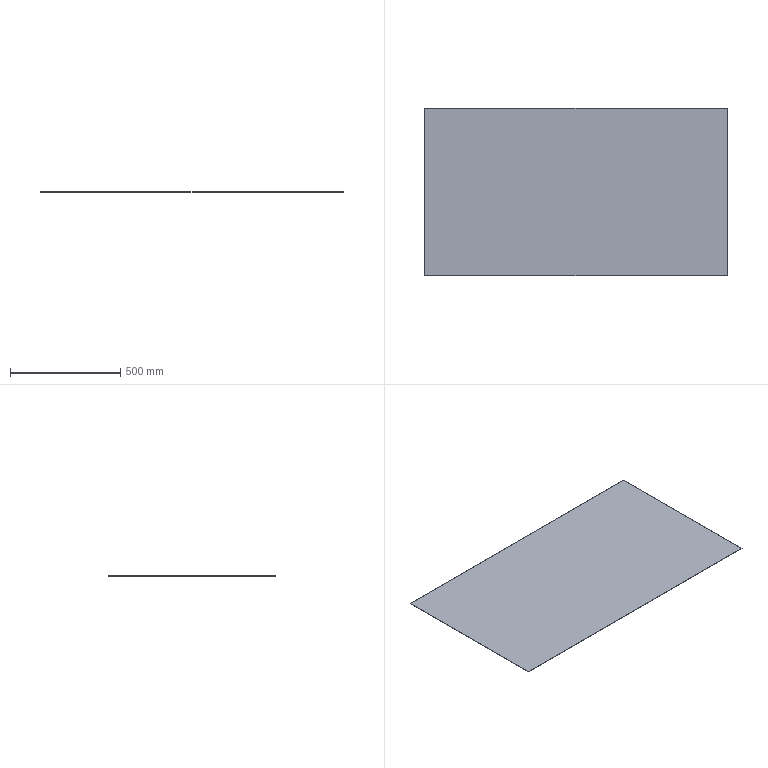Part | SolidWorks | 1 solid | 6 faces | box 1374 x 760 x 1.5 mm | volume 1566360 mm3 | plane 6
STEP:
#1=CARTESIAN_POINT('',(5.,-365.,0.));
#2=VERTEX_POINT('',#1);
#3=CARTESIAN_POINT('',(5.,395.,0.));
#4=VERTEX_POINT('',#3);
#5=CARTESIAN_POINT('',(5.,-365.,0.));
#6=DIRECTION('',(0.,1.,0.));
#7=VECTOR('',#6,1000.);
#8=LINE('',#5,#7);
#9=EDGE_CURVE('',#2,#4,#8,.T.);
#10=ORIENTED_EDGE('',*,*,#9,.T.);
#11=CARTESIAN_POINT('',(5.,395.,1.5));
#12=VERTEX_POINT('',#11);
#13=CARTESIAN_POINT('',(5.,395.,1.5));
#14=DIRECTION('',(0.,0.,-1.));
#15=VECTOR('',#14,1000.);
#16=LINE('',#13,#15);
#17=EDGE_CURVE('',#12,#4,#16,.T.);
#18=ORIENTED_EDGE('',*,*,#17,.F.);
#19=CARTESIAN_POINT('',(5.,-365.,1.5));
#20=VERTEX_POINT('',#19);
#21=CARTESIAN_POINT('',(5.,-365.,1.5));
#22=DIRECTION('',(0.,1.,0.));
#23=VECTOR('',#22,1000.);
#24=LINE('',#21,#23);
#25=EDGE_CURVE('',#20,#12,#24,.T.);
#26=ORIENTED_EDGE('',*,*,#25,.F.);
#27=CARTESIAN_POINT('',(5.,-365.,1.5));
#28=DIRECTION('',(0.,0.,-1.));
#29=VECTOR('',#28,1000.);
#30=LINE('',#27,#29);
#31=EDGE_CURVE('',#20,#2,#30,.T.);
#32=ORIENTED_EDGE('',*,*,#31,.T.);
#33=EDGE_LOOP('',(#10,#18,#26,#32));
#34=FACE_OUTER_BOUND('',#33,.T.);
#35=CARTESIAN_POINT('',(5.,-365.,1.5));
#36=DIRECTION('',(-1.,0.,0.));
#37=DIRECTION('',(0.,0.,1.));
#38=AXIS2_PLACEMENT_3D('',#35,#36,#37);
#39=PLANE('',#38);
#40=ADVANCED_FACE('',(#34),#39,.F.);
#41=CARTESIAN_POINT('',(-1369.,395.,0.));
#42=VERTEX_POINT('',#41);
#43=CARTESIAN_POINT('',(5.,395.,0.));
#44=DIRECTION('',(-1.,0.,0.));
#45=VECTOR('',#44,1000.);
#46=LINE('',#43,#45);
#47=EDGE_CURVE('',#4,#42,#46,.T.);
#48=ORIENTED_EDGE('',*,*,#47,.T.);
#49=CARTESIAN_POINT('',(-1369.,395.,1.5));
#50=VERTEX_POINT('',#49);
#51=CARTESIAN_POINT('',(-1369.,395.,1.5));
#52=DIRECTION('',(0.,0.,-1.));
#53=VECTOR('',#52,1000.);
#54=LINE('',#51,#53);
#55=EDGE_CURVE('',#50,#42,#54,.T.);
#56=ORIENTED_EDGE('',*,*,#55,.F.);
#57=CARTESIAN_POINT('',(5.,395.,1.5));
#58=DIRECTION('',(-1.,0.,0.));
#59=VECTOR('',#58,1000.);
#60=LINE('',#57,#59);
#61=EDGE_CURVE('',#12,#50,#60,.T.);
#62=ORIENTED_EDGE('',*,*,#61,.F.);
#63=ORIENTED_EDGE('',*,*,#17,.T.);
#64=EDGE_LOOP('',(#48,#56,#62,#63));
#65=FACE_OUTER_BOUND('',#64,.T.);
#66=CARTESIAN_POINT('',(5.,395.,1.5));
#67=DIRECTION('',(0.,-1.,0.));
#68=DIRECTION('',(1.,0.,0.));
#69=AXIS2_PLACEMENT_3D('',#66,#67,#68);
#70=PLANE('',#69);
#71=ADVANCED_FACE('',(#65),#70,.F.);
#72=CARTESIAN_POINT('',(-1369.,-365.,0.));
#73=VERTEX_POINT('',#72);
#74=CARTESIAN_POINT('',(-1369.,-365.,0.));
#75=DIRECTION('',(0.,-1.,0.));
#76=VECTOR('',#75,1000.);
#77=LINE('',#74,#76);
#78=EDGE_CURVE('',#42,#73,#77,.T.);
#79=ORIENTED_EDGE('',*,*,#78,.T.);
#80=CARTESIAN_POINT('',(-1369.,-365.,1.5));
#81=VERTEX_POINT('',#80);
#82=CARTESIAN_POINT('',(-1369.,-365.,1.5));
#83=DIRECTION('',(0.,0.,-1.));
#84=VECTOR('',#83,1000.);
#85=LINE('',#82,#84);
#86=EDGE_CURVE('',#81,#73,#85,.T.);
#87=ORIENTED_EDGE('',*,*,#86,.F.);
#88=CARTESIAN_POINT('',(-1369.,-365.,1.5));
#89=DIRECTION('',(0.,-1.,0.));
#90=VECTOR('',#89,1000.);
#91=LINE('',#88,#90);
#92=EDGE_CURVE('',#50,#81,#91,.T.);
#93=ORIENTED_EDGE('',*,*,#92,.F.);
#94=ORIENTED_EDGE('',*,*,#55,.T.);
#95=EDGE_LOOP('',(#79,#87,#93,#94));
#96=FACE_OUTER_BOUND('',#95,.T.);
#97=CARTESIAN_POINT('',(-1369.,-365.,1.5));
#98=DIRECTION('',(1.,0.,0.));
#99=DIRECTION('',(0.,0.,-1.));
#100=AXIS2_PLACEMENT_3D('',#97,#98,#99);
#101=PLANE('',#100);
#102=ADVANCED_FACE('',(#96),#101,.F.);
#103=CARTESIAN_POINT('',(5.,-365.,0.));
#104=DIRECTION('',(1.,0.,0.));
#105=VECTOR('',#104,1000.);
#106=LINE('',#103,#105);
#107=EDGE_CURVE('',#73,#2,#106,.T.);
#108=ORIENTED_EDGE('',*,*,#107,.T.);
#109=ORIENTED_EDGE('',*,*,#31,.F.);
#110=CARTESIAN_POINT('',(5.,-365.,1.5));
#111=DIRECTION('',(1.,0.,0.));
#112=VECTOR('',#111,1000.);
#113=LINE('',#110,#112);
#114=EDGE_CURVE('',#81,#20,#113,.T.);
#115=ORIENTED_EDGE('',*,*,#114,.F.);
#116=ORIENTED_EDGE('',*,*,#86,.T.);
#117=EDGE_LOOP('',(#108,#109,#115,#116));
#118=FACE_OUTER_BOUND('',#117,.T.);
#119=CARTESIAN_POINT('',(5.,-365.,1.5));
#120=DIRECTION('',(0.,1.,0.));
#121=DIRECTION('',(-1.,0.,0.));
#122=AXIS2_PLACEMENT_3D('',#119,#120,#121);
#123=PLANE('',#122);
#124=ADVANCED_FACE('',(#118),#123,.F.);
#125=ORIENTED_EDGE('',*,*,#25,.T.);
#126=ORIENTED_EDGE('',*,*,#61,.T.);
#127=ORIENTED_EDGE('',*,*,#92,.T.);
#128=ORIENTED_EDGE('',*,*,#114,.T.);
#129=EDGE_LOOP('',(#125,#126,#127,#128));
#130=FACE_OUTER_BOUND('',#129,.T.);
#131=CARTESIAN_POINT('',(0.,0.,1.5));
#132=DIRECTION('',(0.,0.,1.));
#133=DIRECTION('',(1.,0.,0.));
#134=AXIS2_PLACEMENT_3D('',#131,#132,#133);
#135=PLANE('',#134);
#136=ADVANCED_FACE('',(#130),#135,.T.);
#137=ORIENTED_EDGE('',*,*,#9,.F.);
#138=ORIENTED_EDGE('',*,*,#107,.F.);
#139=ORIENTED_EDGE('',*,*,#78,.F.);
#140=ORIENTED_EDGE('',*,*,#47,.F.);
#141=EDGE_LOOP('',(#137,#138,#139,#140));
#142=FACE_OUTER_BOUND('',#141,.T.);
#143=CARTESIAN_POINT('',(0.,0.,0.));
#144=DIRECTION('',(0.,0.,1.));
#145=DIRECTION('',(1.,0.,0.));
#146=AXIS2_PLACEMENT_3D('',#143,#144,#145);
#147=PLANE('',#146);
#148=ADVANCED_FACE('',(#142),#147,.F.);
#149=CLOSED_SHELL('',(#40,#71,#102,#124,#136,#148));
#150=MANIFOLD_SOLID_BREP('',#149);
#151=CARTESIAN_POINT('',(0.,0.,0.));
#152=DIRECTION('',(0.,0.,1.));
#153=DIRECTION('',(1.,0.,0.));
#154=AXIS2_PLACEMENT_3D('',#151,#152,#153);
#155=(LENGTH_UNIT()NAMED_UNIT(*)SI_UNIT(.MILLI.,.METRE.));
#156=UNCERTAINTY_MEASURE_WITH_UNIT(LENGTH_MEASURE(0.00001),#155,'','');
#157=(NAMED_UNIT(*)PLANE_ANGLE_UNIT()SI_UNIT($,.RADIAN.));
#158=(NAMED_UNIT(*)SI_UNIT($,.STERADIAN.)SOLID_ANGLE_UNIT());
#159=(GEOMETRIC_REPRESENTATION_CONTEXT(3)GLOBAL_UNCERTAINTY_ASSIGNED_CONTEXT((#156))GLOBAL_UNIT_ASSIGNED_CONTEXT((#155,#157,#158))REPRESENTATION_CONTEXT('',''));
#160=ADVANCED_BREP_SHAPE_REPRESENTATION('',(#150,#154),#159);